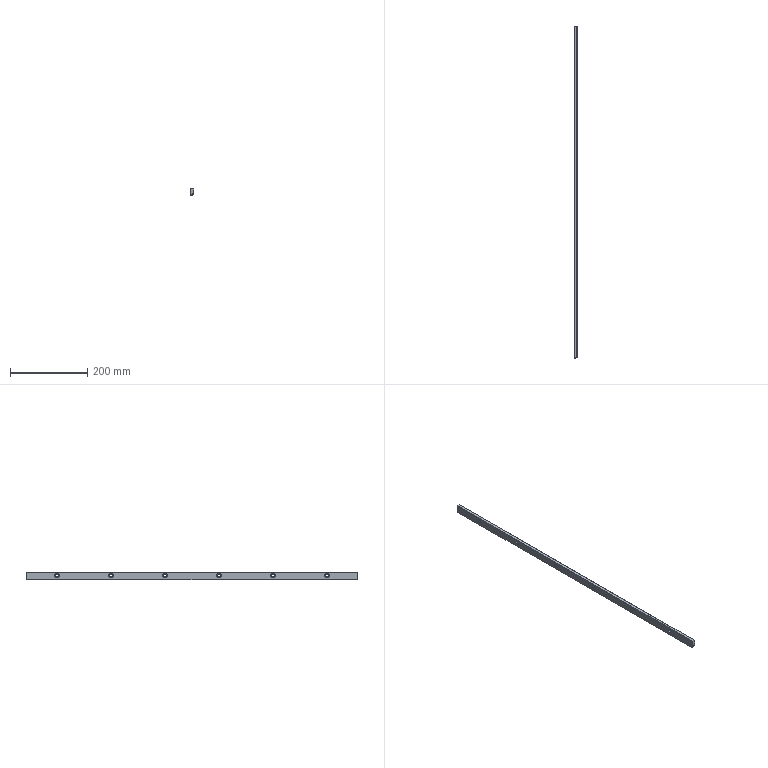Part | STEP file | PN_0001 06B Side Guide Chain Support Block L860 | 1 solid | 48 faces | box 9 x 860 x 20.4 mm | volume 137278 mm3 | cylinder 30 | plane 18 | commonest cylinder face diameters 6.5 x12 12 x12 3 x6